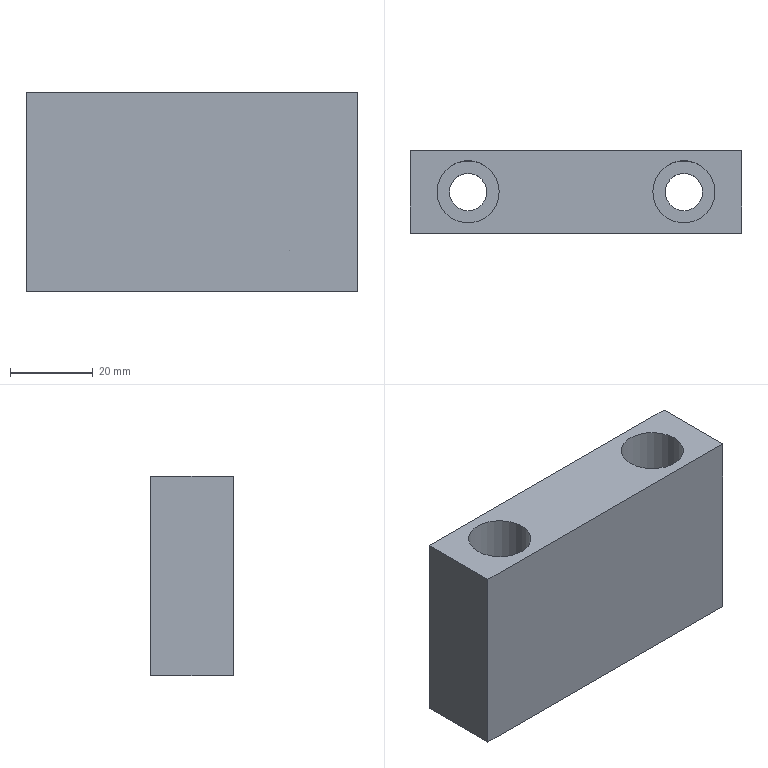Part | STEP file | gslz 2016.10.28-13_id498_x_t | 1 solid | 12 faces | box 80 x 20 x 48 mm | volume 65038 mm3 | plane 8 | cylinder 4 | commonest cylinder face diameters 9 x2 15 x2
STEP:
#1=CARTESIAN_POINT('',(0.,0.,0.));
#2=DIRECTION('',(0.,0.,1.));
#3=DIRECTION('',(1.,0.,0.));
#4=AXIS2_PLACEMENT_3D('',#1,#2,#3);
#5=CARTESIAN_POINT('',(-745.014,-46.466,0.));
#6=VERTEX_POINT('',#5);
#7=CARTESIAN_POINT('',(-737.514,-46.466,0.));
#8=DIRECTION('',(0.,0.,-1.));
#9=DIRECTION('',(-1.,0.,0.));
#10=AXIS2_PLACEMENT_3D('',#7,#8,#9);
#11=CIRCLE('',#10,7.5);
#12=CARTESIAN_POINT('',(-834.,82.556,0.));
#13=DIRECTION('',(0.,0.,-1.));
#14=DIRECTION('',(-1.,0.,0.));
#15=AXIS2_PLACEMENT_3D('',#12,#13,#14);
#16=PLANE('',#15);
#17=CARTESIAN_POINT('',(-96.486,-129.022));
#18=DIRECTION('',(1.,0.));
#19=AXIS2_PLACEMENT_2D('',#17,#18);
#20=CIRCLE('',#19,7.5);
#21=(GEOMETRIC_REPRESENTATION_CONTEXT(2)PARAMETRIC_REPRESENTATION_CONTEXT()REPRESENTATION_CONTEXT('',''));
#22=DEFINITIONAL_REPRESENTATION('',(#20),#21);
#23=PCURVE('',#16,#22);
#24=CARTESIAN_POINT('',(-737.514,-46.466,0.));
#25=DIRECTION('',(0.,0.,-1.));
#26=DIRECTION('',(-1.,0.,0.));
#27=AXIS2_PLACEMENT_3D('',#24,#25,#26);
#28=CYLINDRICAL_SURFACE('',#27,7.5);
#29=CARTESIAN_POINT('',(0.,0.));
#30=DIRECTION('',(1.,0.));
#31=VECTOR('',#30,1.);
#32=LINE('',#29,#31);
#33=(GEOMETRIC_REPRESENTATION_CONTEXT(2)PARAMETRIC_REPRESENTATION_CONTEXT()REPRESENTATION_CONTEXT('',''));
#34=DEFINITIONAL_REPRESENTATION('',(#32),#33);
#35=PCURVE('',#28,#34);
#36=SURFACE_CURVE('',#11,(#23,#35),.PCURVE_S1.);
#37=EDGE_CURVE('',#6,#6,#36,.T.);
#38=ORIENTED_EDGE('',*,*,#37,.T.);
#39=EDGE_LOOP('',(#38));
#40=FACE_BOUND('',#39,.T.);
#41=CARTESIAN_POINT('',(-797.014,-46.466,0.));
#42=VERTEX_POINT('',#41);
#43=CARTESIAN_POINT('',(-789.514,-46.466,0.));
#44=DIRECTION('',(0.,0.,-1.));
#45=DIRECTION('',(-1.,0.,0.));
#46=AXIS2_PLACEMENT_3D('',#43,#44,#45);
#47=CIRCLE('',#46,7.5);
#48=CARTESIAN_POINT('',(-44.486,-129.022));
#49=DIRECTION('',(1.,0.));
#50=AXIS2_PLACEMENT_2D('',#48,#49);
#51=CIRCLE('',#50,7.5);
#52=(GEOMETRIC_REPRESENTATION_CONTEXT(2)PARAMETRIC_REPRESENTATION_CONTEXT()REPRESENTATION_CONTEXT('',''));
#53=DEFINITIONAL_REPRESENTATION('',(#51),#52);
#54=PCURVE('',#16,#53);
#55=CARTESIAN_POINT('',(-789.514,-46.466,0.));
#56=DIRECTION('',(0.,0.,-1.));
#57=DIRECTION('',(-1.,0.,0.));
#58=AXIS2_PLACEMENT_3D('',#55,#56,#57);
#59=CYLINDRICAL_SURFACE('',#58,7.5);
#60=CARTESIAN_POINT('',(0.,0.));
#61=DIRECTION('',(1.,0.));
#62=VECTOR('',#61,1.);
#63=LINE('',#60,#62);
#64=(GEOMETRIC_REPRESENTATION_CONTEXT(2)PARAMETRIC_REPRESENTATION_CONTEXT()REPRESENTATION_CONTEXT('',''));
#65=DEFINITIONAL_REPRESENTATION('',(#63),#64);
#66=PCURVE('',#59,#65);
#67=SURFACE_CURVE('',#47,(#54,#66),.PCURVE_S1.);
#68=EDGE_CURVE('',#42,#42,#67,.T.);
#69=ORIENTED_EDGE('',*,*,#68,.T.);
#70=EDGE_LOOP('',(#69));
#71=FACE_BOUND('',#70,.T.);
#72=CARTESIAN_POINT('',(-723.514,-56.466,0.));
#73=VERTEX_POINT('',#72);
#74=CARTESIAN_POINT('',(-803.514,-56.466,0.));
#75=VERTEX_POINT('',#74);
#76=CARTESIAN_POINT('',(-763.514,-56.466,0.));
#77=DIRECTION('',(-1.,0.,0.));
#78=VECTOR('',#77,1.);
#79=LINE('',#76,#78);
#80=CARTESIAN_POINT('',(-70.486,-139.022));
#81=DIRECTION('',(1.,0.));
#82=VECTOR('',#81,1.);
#83=LINE('',#80,#82);
#84=(GEOMETRIC_REPRESENTATION_CONTEXT(2)PARAMETRIC_REPRESENTATION_CONTEXT()REPRESENTATION_CONTEXT('',''));
#85=DEFINITIONAL_REPRESENTATION('',(#83),#84);
#86=PCURVE('',#16,#85);
#87=CARTESIAN_POINT('',(-763.514,-56.466,-13.75));
#88=DIRECTION('',(0.,-1.,0.));
#89=DIRECTION('',(0.,0.,-1.));
#90=AXIS2_PLACEMENT_3D('',#87,#88,#89);
#91=PLANE('',#90);
#92=CARTESIAN_POINT('',(-13.75,0.));
#93=DIRECTION('',(0.,-1.));
#94=VECTOR('',#93,1.);
#95=LINE('',#92,#94);
#96=(GEOMETRIC_REPRESENTATION_CONTEXT(2)PARAMETRIC_REPRESENTATION_CONTEXT()REPRESENTATION_CONTEXT('',''));
#97=DEFINITIONAL_REPRESENTATION('',(#95),#96);
#98=PCURVE('',#91,#97);
#99=SURFACE_CURVE('',#79,(#86,#98),.PCURVE_S1.);
#100=EDGE_CURVE('',#73,#75,#99,.T.);
#101=ORIENTED_EDGE('',*,*,#100,.F.);
#102=CARTESIAN_POINT('',(-723.514,-36.466,0.));
#103=VERTEX_POINT('',#102);
#104=CARTESIAN_POINT('',(-723.514,-55.466,0.));
#105=DIRECTION('',(0.,-1.,0.));
#106=VECTOR('',#105,1.);
#107=LINE('',#104,#106);
#108=CARTESIAN_POINT('',(-110.486,-138.022));
#109=DIRECTION('',(0.,-1.));
#110=VECTOR('',#109,1.);
#111=LINE('',#108,#110);
#112=(GEOMETRIC_REPRESENTATION_CONTEXT(2)PARAMETRIC_REPRESENTATION_CONTEXT()REPRESENTATION_CONTEXT('',''));
#113=DEFINITIONAL_REPRESENTATION('',(#111),#112);
#114=PCURVE('',#16,#113);
#115=CARTESIAN_POINT('',(-723.514,-55.466,-13.75));
#116=DIRECTION('',(1.,0.,0.));
#117=DIRECTION('',(0.,0.,-1.));
#118=AXIS2_PLACEMENT_3D('',#115,#116,#117);
#119=PLANE('',#118);
#120=CARTESIAN_POINT('',(-13.75,0.));
#121=DIRECTION('',(0.,-1.));
#122=VECTOR('',#121,1.);
#123=LINE('',#120,#122);
#124=(GEOMETRIC_REPRESENTATION_CONTEXT(2)PARAMETRIC_REPRESENTATION_CONTEXT()REPRESENTATION_CONTEXT('',''));
#125=DEFINITIONAL_REPRESENTATION('',(#123),#124);
#126=PCURVE('',#119,#125);
#127=SURFACE_CURVE('',#107,(#114,#126),.PCURVE_S1.);
#128=EDGE_CURVE('',#103,#73,#127,.T.);
#129=ORIENTED_EDGE('',*,*,#128,.F.);
#130=CARTESIAN_POINT('',(-803.514,-36.466,0.));
#131=VERTEX_POINT('',#130);
#132=CARTESIAN_POINT('',(-763.514,-36.466,0.));
#133=DIRECTION('',(1.,0.,0.));
#134=VECTOR('',#133,1.);
#135=LINE('',#132,#134);
#136=CARTESIAN_POINT('',(-70.486,-119.022));
#137=DIRECTION('',(-1.,0.));
#138=VECTOR('',#137,1.);
#139=LINE('',#136,#138);
#140=(GEOMETRIC_REPRESENTATION_CONTEXT(2)PARAMETRIC_REPRESENTATION_CONTEXT()REPRESENTATION_CONTEXT('',''));
#141=DEFINITIONAL_REPRESENTATION('',(#139),#140);
#142=PCURVE('',#16,#141);
#143=CARTESIAN_POINT('',(-763.514,-36.466,-13.75));
#144=DIRECTION('',(0.,1.,0.));
#145=DIRECTION('',(0.,0.,1.));
#146=AXIS2_PLACEMENT_3D('',#143,#144,#145);
#147=PLANE('',#146);
#148=CARTESIAN_POINT('',(13.75,0.));
#149=DIRECTION('',(0.,1.));
#150=VECTOR('',#149,1.);
#151=LINE('',#148,#150);
#152=(GEOMETRIC_REPRESENTATION_CONTEXT(2)PARAMETRIC_REPRESENTATION_CONTEXT()REPRESENTATION_CONTEXT('',''));
#153=DEFINITIONAL_REPRESENTATION('',(#151),#152);
#154=PCURVE('',#147,#153);
#155=SURFACE_CURVE('',#135,(#142,#154),.PCURVE_S1.);
#156=EDGE_CURVE('',#131,#103,#155,.T.);
#157=ORIENTED_EDGE('',*,*,#156,.F.);
#158=CARTESIAN_POINT('',(-803.514,-55.466,0.));
#159=DIRECTION('',(0.,1.,0.));
#160=VECTOR('',#159,1.);
#161=LINE('',#158,#160);
#162=CARTESIAN_POINT('',(-30.486,-138.022));
#163=DIRECTION('',(0.,1.));
#164=VECTOR('',#163,1.);
#165=LINE('',#162,#164);
#166=(GEOMETRIC_REPRESENTATION_CONTEXT(2)PARAMETRIC_REPRESENTATION_CONTEXT()REPRESENTATION_CONTEXT('',''));
#167=DEFINITIONAL_REPRESENTATION('',(#165),#166);
#168=PCURVE('',#16,#167);
#169=CARTESIAN_POINT('',(-803.514,-55.466,-13.75));
#170=DIRECTION('',(-1.,0.,0.));
#171=DIRECTION('',(0.,0.,1.));
#172=AXIS2_PLACEMENT_3D('',#169,#170,#171);
#173=PLANE('',#172);
#174=CARTESIAN_POINT('',(13.75,0.));
#175=DIRECTION('',(0.,1.));
#176=VECTOR('',#175,1.);
#177=LINE('',#174,#176);
#178=(GEOMETRIC_REPRESENTATION_CONTEXT(2)PARAMETRIC_REPRESENTATION_CONTEXT()REPRESENTATION_CONTEXT('',''));
#179=DEFINITIONAL_REPRESENTATION('',(#177),#178);
#180=PCURVE('',#173,#179);
#181=SURFACE_CURVE('',#161,(#168,#180),.PCURVE_S1.);
#182=EDGE_CURVE('',#75,#131,#181,.T.);
#183=ORIENTED_EDGE('',*,*,#182,.F.);
#184=EDGE_LOOP('',(#101,#129,#157,#183));
#185=FACE_BOUND('',#184,.T.);
#186=ADVANCED_FACE('',(#40,#71,#185),#16,.F.);
#187=CARTESIAN_POINT('',(-723.514,-56.466,-48.));
#188=VERTEX_POINT('',#187);
#189=CARTESIAN_POINT('',(-723.514,-56.466,-13.75));
#190=DIRECTION('',(0.,0.,1.));
#191=VECTOR('',#190,1.);
#192=LINE('',#189,#191);
#193=CARTESIAN_POINT('',(0.,40.));
#194=DIRECTION('',(-1.,0.));
#195=VECTOR('',#194,1.);
#196=LINE('',#193,#195);
#197=(GEOMETRIC_REPRESENTATION_CONTEXT(2)PARAMETRIC_REPRESENTATION_CONTEXT()REPRESENTATION_CONTEXT('',''));
#198=DEFINITIONAL_REPRESENTATION('',(#196),#197);
#199=PCURVE('',#91,#198);
#200=CARTESIAN_POINT('',(0.,-1.));
#201=DIRECTION('',(-1.,0.));
#202=VECTOR('',#201,1.);
#203=LINE('',#200,#202);
#204=(GEOMETRIC_REPRESENTATION_CONTEXT(2)PARAMETRIC_REPRESENTATION_CONTEXT()REPRESENTATION_CONTEXT('',''));
#205=DEFINITIONAL_REPRESENTATION('',(#203),#204);
#206=PCURVE('',#119,#205);
#207=SURFACE_CURVE('',#192,(#199,#206),.PCURVE_S1.);
#208=EDGE_CURVE('',#188,#73,#207,.T.);
#209=ORIENTED_EDGE('',*,*,#208,.T.);
#210=ORIENTED_EDGE('',*,*,#100,.T.);
#211=CARTESIAN_POINT('',(-803.514,-56.466,-48.));
#212=VERTEX_POINT('',#211);
#213=CARTESIAN_POINT('',(-803.514,-56.466,-13.75));
#214=DIRECTION('',(0.,0.,1.));
#215=VECTOR('',#214,1.);
#216=LINE('',#213,#215);
#217=CARTESIAN_POINT('',(0.,-40.));
#218=DIRECTION('',(-1.,0.));
#219=VECTOR('',#218,1.);
#220=LINE('',#217,#219);
#221=(GEOMETRIC_REPRESENTATION_CONTEXT(2)PARAMETRIC_REPRESENTATION_CONTEXT()REPRESENTATION_CONTEXT('',''));
#222=DEFINITIONAL_REPRESENTATION('',(#220),#221);
#223=PCURVE('',#91,#222);
#224=CARTESIAN_POINT('',(0.,-1.));
#225=DIRECTION('',(1.,0.));
#226=VECTOR('',#225,1.);
#227=LINE('',#224,#226);
#228=(GEOMETRIC_REPRESENTATION_CONTEXT(2)PARAMETRIC_REPRESENTATION_CONTEXT()REPRESENTATION_CONTEXT('',''));
#229=DEFINITIONAL_REPRESENTATION('',(#227),#228);
#230=PCURVE('',#173,#229);
#231=SURFACE_CURVE('',#216,(#223,#230),.PCURVE_S1.);
#232=EDGE_CURVE('',#212,#75,#231,.T.);
#233=ORIENTED_EDGE('',*,*,#232,.F.);
#234=CARTESIAN_POINT('',(-763.514,-56.466,-48.));
#235=DIRECTION('',(1.,0.,0.));
#236=VECTOR('',#235,1.);
#237=LINE('',#234,#236);
#238=CARTESIAN_POINT('',(34.25,0.));
#239=DIRECTION('',(0.,1.));
#240=VECTOR('',#239,1.);
#241=LINE('',#238,#240);
#242=(GEOMETRIC_REPRESENTATION_CONTEXT(2)PARAMETRIC_REPRESENTATION_CONTEXT()REPRESENTATION_CONTEXT('',''));
#243=DEFINITIONAL_REPRESENTATION('',(#241),#242);
#244=PCURVE('',#91,#243);
#245=CARTESIAN_POINT('',(-834.,82.556,-48.));
#246=DIRECTION('',(0.,0.,-1.));
#247=DIRECTION('',(-1.,0.,0.));
#248=AXIS2_PLACEMENT_3D('',#245,#246,#247);
#249=PLANE('',#248);
#250=CARTESIAN_POINT('',(-70.486,-139.022));
#251=DIRECTION('',(-1.,0.));
#252=VECTOR('',#251,1.);
#253=LINE('',#250,#252);
#254=(GEOMETRIC_REPRESENTATION_CONTEXT(2)PARAMETRIC_REPRESENTATION_CONTEXT()REPRESENTATION_CONTEXT('',''));
#255=DEFINITIONAL_REPRESENTATION('',(#253),#254);
#256=PCURVE('',#249,#255);
#257=SURFACE_CURVE('',#237,(#244,#256),.PCURVE_S1.);
#258=EDGE_CURVE('',#212,#188,#257,.T.);
#259=ORIENTED_EDGE('',*,*,#258,.T.);
#260=EDGE_LOOP('',(#209,#210,#233,#259));
#261=FACE_BOUND('',#260,.T.);
#262=ADVANCED_FACE('',(#261),#91,.T.);
#263=ORIENTED_EDGE('',*,*,#232,.T.);
#264=ORIENTED_EDGE('',*,*,#182,.T.);
#265=CARTESIAN_POINT('',(-803.514,-36.466,-48.));
#266=VERTEX_POINT('',#265);
#267=CARTESIAN_POINT('',(-803.514,-36.466,-13.75));
#268=DIRECTION('',(0.,0.,1.));
#269=VECTOR('',#268,1.);
#270=LINE('',#267,#269);
#271=CARTESIAN_POINT('',(0.,19.));
#272=DIRECTION('',(1.,0.));
#273=VECTOR('',#272,1.);
#274=LINE('',#271,#273);
#275=(GEOMETRIC_REPRESENTATION_CONTEXT(2)PARAMETRIC_REPRESENTATION_CONTEXT()REPRESENTATION_CONTEXT('',''));
#276=DEFINITIONAL_REPRESENTATION('',(#274),#275);
#277=PCURVE('',#173,#276);
#278=CARTESIAN_POINT('',(0.,-40.));
#279=DIRECTION('',(1.,0.));
#280=VECTOR('',#279,1.);
#281=LINE('',#278,#280);
#282=(GEOMETRIC_REPRESENTATION_CONTEXT(2)PARAMETRIC_REPRESENTATION_CONTEXT()REPRESENTATION_CONTEXT('',''));
#283=DEFINITIONAL_REPRESENTATION('',(#281),#282);
#284=PCURVE('',#147,#283);
#285=SURFACE_CURVE('',#270,(#277,#284),.PCURVE_S1.);
#286=EDGE_CURVE('',#266,#131,#285,.T.);
#287=ORIENTED_EDGE('',*,*,#286,.F.);
#288=CARTESIAN_POINT('',(-803.514,-55.466,-48.));
#289=DIRECTION('',(0.,-1.,0.));
#290=VECTOR('',#289,1.);
#291=LINE('',#288,#290);
#292=CARTESIAN_POINT('',(-34.25,0.));
#293=DIRECTION('',(0.,-1.));
#294=VECTOR('',#293,1.);
#295=LINE('',#292,#294);
#296=(GEOMETRIC_REPRESENTATION_CONTEXT(2)PARAMETRIC_REPRESENTATION_CONTEXT()REPRESENTATION_CONTEXT('',''));
#297=DEFINITIONAL_REPRESENTATION('',(#295),#296);
#298=PCURVE('',#173,#297);
#299=CARTESIAN_POINT('',(-30.486,-138.022));
#300=DIRECTION('',(0.,-1.));
#301=VECTOR('',#300,1.);
#302=LINE('',#299,#301);
#303=(GEOMETRIC_REPRESENTATION_CONTEXT(2)PARAMETRIC_REPRESENTATION_CONTEXT()REPRESENTATION_CONTEXT('',''));
#304=DEFINITIONAL_REPRESENTATION('',(#302),#303);
#305=PCURVE('',#249,#304);
#306=SURFACE_CURVE('',#291,(#298,#305),.PCURVE_S1.);
#307=EDGE_CURVE('',#266,#212,#306,.T.);
#308=ORIENTED_EDGE('',*,*,#307,.T.);
#309=EDGE_LOOP('',(#263,#264,#287,#308));
#310=FACE_BOUND('',#309,.T.);
#311=ADVANCED_FACE('',(#310),#173,.T.);
#312=ORIENTED_EDGE('',*,*,#286,.T.);
#313=ORIENTED_EDGE('',*,*,#156,.T.);
#314=CARTESIAN_POINT('',(-723.514,-36.466,-48.));
#315=VERTEX_POINT('',#314);
#316=CARTESIAN_POINT('',(-723.514,-36.466,-13.75));
#317=DIRECTION('',(0.,0.,1.));
#318=VECTOR('',#317,1.);
#319=LINE('',#316,#318);
#320=CARTESIAN_POINT('',(0.,40.));
#321=DIRECTION('',(1.,0.));
#322=VECTOR('',#321,1.);
#323=LINE('',#320,#322);
#324=(GEOMETRIC_REPRESENTATION_CONTEXT(2)PARAMETRIC_REPRESENTATION_CONTEXT()REPRESENTATION_CONTEXT('',''));
#325=DEFINITIONAL_REPRESENTATION('',(#323),#324);
#326=PCURVE('',#147,#325);
#327=CARTESIAN_POINT('',(0.,19.));
#328=DIRECTION('',(-1.,0.));
#329=VECTOR('',#328,1.);
#330=LINE('',#327,#329);
#331=(GEOMETRIC_REPRESENTATION_CONTEXT(2)PARAMETRIC_REPRESENTATION_CONTEXT()REPRESENTATION_CONTEXT('',''));
#332=DEFINITIONAL_REPRESENTATION('',(#330),#331);
#333=PCURVE('',#119,#332);
#334=SURFACE_CURVE('',#319,(#326,#333),.PCURVE_S1.);
#335=EDGE_CURVE('',#315,#103,#334,.T.);
#336=ORIENTED_EDGE('',*,*,#335,.F.);
#337=CARTESIAN_POINT('',(-763.514,-36.466,-48.));
#338=DIRECTION('',(-1.,0.,0.));
#339=VECTOR('',#338,1.);
#340=LINE('',#337,#339);
#341=CARTESIAN_POINT('',(-34.25,0.));
#342=DIRECTION('',(0.,-1.));
#343=VECTOR('',#342,1.);
#344=LINE('',#341,#343);
#345=(GEOMETRIC_REPRESENTATION_CONTEXT(2)PARAMETRIC_REPRESENTATION_CONTEXT()REPRESENTATION_CONTEXT('',''));
#346=DEFINITIONAL_REPRESENTATION('',(#344),#345);
#347=PCURVE('',#147,#346);
#348=CARTESIAN_POINT('',(-70.486,-119.022));
#349=DIRECTION('',(1.,0.));
#350=VECTOR('',#349,1.);
#351=LINE('',#348,#350);
#352=(GEOMETRIC_REPRESENTATION_CONTEXT(2)PARAMETRIC_REPRESENTATION_CONTEXT()REPRESENTATION_CONTEXT('',''));
#353=DEFINITIONAL_REPRESENTATION('',(#351),#352);
#354=PCURVE('',#249,#353);
#355=SURFACE_CURVE('',#340,(#347,#354),.PCURVE_S1.);
#356=EDGE_CURVE('',#315,#266,#355,.T.);
#357=ORIENTED_EDGE('',*,*,#356,.T.);
#358=EDGE_LOOP('',(#312,#313,#336,#357));
#359=FACE_BOUND('',#358,.T.);
#360=ADVANCED_FACE('',(#359),#147,.T.);
#361=CARTESIAN_POINT('',(-742.014,-46.466,-48.));
#362=VERTEX_POINT('',#361);
#363=CARTESIAN_POINT('',(-737.514,-46.466,-48.));
#364=DIRECTION('',(0.,0.,-1.));
#365=DIRECTION('',(-1.,0.,0.));
#366=AXIS2_PLACEMENT_3D('',#363,#364,#365);
#367=CIRCLE('',#366,4.5);
#368=CARTESIAN_POINT('',(-96.486,-129.022));
#369=DIRECTION('',(1.,0.));
#370=AXIS2_PLACEMENT_2D('',#368,#369);
#371=CIRCLE('',#370,4.5);
#372=(GEOMETRIC_REPRESENTATION_CONTEXT(2)PARAMETRIC_REPRESENTATION_CONTEXT()REPRESENTATION_CONTEXT('',''));
#373=DEFINITIONAL_REPRESENTATION('',(#371),#372);
#374=PCURVE('',#249,#373);
#375=CARTESIAN_POINT('',(-737.514,-46.466,-150.));
#376=DIRECTION('',(0.,0.,-1.));
#377=DIRECTION('',(-1.,0.,0.));
#378=AXIS2_PLACEMENT_3D('',#375,#376,#377);
#379=CYLINDRICAL_SURFACE('',#378,4.5);
#380=CARTESIAN_POINT('',(0.,-102.));
#381=DIRECTION('',(1.,0.));
#382=VECTOR('',#381,1.);
#383=LINE('',#380,#382);
#384=(GEOMETRIC_REPRESENTATION_CONTEXT(2)PARAMETRIC_REPRESENTATION_CONTEXT()REPRESENTATION_CONTEXT('',''));
#385=DEFINITIONAL_REPRESENTATION('',(#383),#384);
#386=PCURVE('',#379,#385);
#387=SURFACE_CURVE('',#367,(#374,#386),.PCURVE_S1.);
#388=EDGE_CURVE('',#362,#362,#387,.T.);
#389=ORIENTED_EDGE('',*,*,#388,.F.);
#390=EDGE_LOOP('',(#389));
#391=FACE_BOUND('',#390,.T.);
#392=CARTESIAN_POINT('',(-794.014,-46.466,-48.));
#393=VERTEX_POINT('',#392);
#394=CARTESIAN_POINT('',(-789.514,-46.466,-48.));
#395=DIRECTION('',(0.,0.,-1.));
#396=DIRECTION('',(-1.,0.,0.));
#397=AXIS2_PLACEMENT_3D('',#394,#395,#396);
#398=CIRCLE('',#397,4.5);
#399=CARTESIAN_POINT('',(-44.486,-129.022));
#400=DIRECTION('',(1.,0.));
#401=AXIS2_PLACEMENT_2D('',#399,#400);
#402=CIRCLE('',#401,4.5);
#403=(GEOMETRIC_REPRESENTATION_CONTEXT(2)PARAMETRIC_REPRESENTATION_CONTEXT()REPRESENTATION_CONTEXT('',''));
#404=DEFINITIONAL_REPRESENTATION('',(#402),#403);
#405=PCURVE('',#249,#404);
#406=CARTESIAN_POINT('',(-789.514,-46.466,-150.));
#407=DIRECTION('',(0.,0.,-1.));
#408=DIRECTION('',(-1.,0.,0.));
#409=AXIS2_PLACEMENT_3D('',#406,#407,#408);
#410=CYLINDRICAL_SURFACE('',#409,4.5);
#411=CARTESIAN_POINT('',(0.,-102.));
#412=DIRECTION('',(1.,0.));
#413=VECTOR('',#412,1.);
#414=LINE('',#411,#413);
#415=(GEOMETRIC_REPRESENTATION_CONTEXT(2)PARAMETRIC_REPRESENTATION_CONTEXT()REPRESENTATION_CONTEXT('',''));
#416=DEFINITIONAL_REPRESENTATION('',(#414),#415);
#417=PCURVE('',#410,#416);
#418=SURFACE_CURVE('',#398,(#405,#417),.PCURVE_S1.);
#419=EDGE_CURVE('',#393,#393,#418,.T.);
#420=ORIENTED_EDGE('',*,*,#419,.F.);
#421=EDGE_LOOP('',(#420));
#422=FACE_BOUND('',#421,.T.);
#423=CARTESIAN_POINT('',(-723.514,-55.466,-48.));
#424=DIRECTION('',(0.,1.,0.));
#425=VECTOR('',#424,1.);
#426=LINE('',#423,#425);
#427=CARTESIAN_POINT('',(-110.486,-138.022));
#428=DIRECTION('',(0.,1.));
#429=VECTOR('',#428,1.);
#430=LINE('',#427,#429);
#431=(GEOMETRIC_REPRESENTATION_CONTEXT(2)PARAMETRIC_REPRESENTATION_CONTEXT()REPRESENTATION_CONTEXT('',''));
#432=DEFINITIONAL_REPRESENTATION('',(#430),#431);
#433=PCURVE('',#249,#432);
#434=CARTESIAN_POINT('',(34.25,0.));
#435=DIRECTION('',(0.,1.));
#436=VECTOR('',#435,1.);
#437=LINE('',#434,#436);
#438=(GEOMETRIC_REPRESENTATION_CONTEXT(2)PARAMETRIC_REPRESENTATION_CONTEXT()REPRESENTATION_CONTEXT('',''));
#439=DEFINITIONAL_REPRESENTATION('',(#437),#438);
#440=PCURVE('',#119,#439);
#441=SURFACE_CURVE('',#426,(#433,#440),.PCURVE_S1.);
#442=EDGE_CURVE('',#188,#315,#441,.T.);
#443=ORIENTED_EDGE('',*,*,#442,.F.);
#444=ORIENTED_EDGE('',*,*,#258,.F.);
#445=ORIENTED_EDGE('',*,*,#307,.F.);
#446=ORIENTED_EDGE('',*,*,#356,.F.);
#447=EDGE_LOOP('',(#443,#444,#445,#446));
#448=FACE_BOUND('',#447,.T.);
#449=ADVANCED_FACE('',(#391,#422,#448),#249,.T.);
#450=ORIENTED_EDGE('',*,*,#442,.T.);
#451=ORIENTED_EDGE('',*,*,#335,.T.);
#452=ORIENTED_EDGE('',*,*,#128,.T.);
#453=ORIENTED_EDGE('',*,*,#208,.F.);
#454=EDGE_LOOP('',(#450,#451,#452,#453));
#455=FACE_BOUND('',#454,.T.);
#456=ADVANCED_FACE('',(#455),#119,.T.);
#457=ORIENTED_EDGE('',*,*,#419,.F.);
#458=CARTESIAN_POINT('',(-794.014,-46.466,-25.));
#459=VERTEX_POINT('',#458);
#460=CARTESIAN_POINT('',(-794.014,-46.466,-25.));
#461=CARTESIAN_POINT('',(-794.014,-46.466,-48.));
#462=B_SPLINE_CURVE_WITH_KNOTS('',1,(#460,#461),.UNSPECIFIED.,.F.,.F.,(2,2),(-125.,-102.),.PIECEWISE_BEZIER_KNOTS.);
#463=CARTESIAN_POINT('',(0.,0.));
#464=DIRECTION('',(0.,1.));
#465=VECTOR('',#464,1.);
#466=LINE('',#463,#465);
#467=(GEOMETRIC_REPRESENTATION_CONTEXT(2)PARAMETRIC_REPRESENTATION_CONTEXT()REPRESENTATION_CONTEXT('',''));
#468=DEFINITIONAL_REPRESENTATION('',(#466),#467);
#469=PCURVE('',#410,#468);
#470=CARTESIAN_POINT('',(6.283,0.));
#471=DIRECTION('',(0.,1.));
#472=VECTOR('',#471,1.);
#473=LINE('',#470,#472);
#474=(GEOMETRIC_REPRESENTATION_CONTEXT(2)PARAMETRIC_REPRESENTATION_CONTEXT()REPRESENTATION_CONTEXT('',''));
#475=DEFINITIONAL_REPRESENTATION('',(#473),#474);
#476=PCURVE('',#410,#475);
#477=SEAM_CURVE('',#462,(#469,#476),.PCURVE_S1.);
#478=EDGE_CURVE('',#459,#393,#477,.T.);
#479=ORIENTED_EDGE('',*,*,#478,.F.);
#480=CARTESIAN_POINT('',(-789.514,-46.466,-25.));
#481=DIRECTION('',(0.,0.,1.));
#482=DIRECTION('',(-1.,0.,0.));
#483=AXIS2_PLACEMENT_3D('',#480,#481,#482);
#484=CIRCLE('',#483,4.5);
#485=CARTESIAN_POINT('',(6.283,-125.));
#486=DIRECTION('',(-1.,0.));
#487=VECTOR('',#486,1.);
#488=LINE('',#485,#487);
#489=(GEOMETRIC_REPRESENTATION_CONTEXT(2)PARAMETRIC_REPRESENTATION_CONTEXT()REPRESENTATION_CONTEXT('',''));
#490=DEFINITIONAL_REPRESENTATION('',(#488),#489);
#491=PCURVE('',#410,#490);
#492=CARTESIAN_POINT('',(-789.514,-46.466,-25.));
#493=DIRECTION('',(0.,0.,-1.));
#494=DIRECTION('',(-1.,0.,0.));
#495=AXIS2_PLACEMENT_3D('',#492,#493,#494);
#496=PLANE('',#495);
#497=CARTESIAN_POINT('',(4.5,0.));
#498=CARTESIAN_POINT('',(4.5,-7.794));
#499=CARTESIAN_POINT('',(-2.25,-3.897));
#500=CARTESIAN_POINT('',(-9.,0.));
#501=CARTESIAN_POINT('',(-2.25,3.897));
#502=CARTESIAN_POINT('',(4.5,7.794));
#503=CARTESIAN_POINT('',(4.5,0.));
#504=(BOUNDED_CURVE()B_SPLINE_CURVE(2,(#497,#498,#499,#500,#501,#502,#503),.UNSPECIFIED.,.T.,.F.)B_SPLINE_CURVE_WITH_KNOTS((1,2,2,2,2,1),(-2.094,0.,2.094,4.189,6.283,8.378),.UNSPECIFIED.)CURVE()GEOMETRIC_REPRESENTATION_ITEM()RATIONAL_B_SPLINE_CURVE((1.,0.5,1.,0.5,1.,0.5,1.))REPRESENTATION_ITEM(''));
#505=(GEOMETRIC_REPRESENTATION_CONTEXT(2)PARAMETRIC_REPRESENTATION_CONTEXT()REPRESENTATION_CONTEXT('',''));
#506=DEFINITIONAL_REPRESENTATION('',(#504),#505);
#507=PCURVE('',#496,#506);
#508=SURFACE_CURVE('',#484,(#491,#507),.PCURVE_S1.);
#509=EDGE_CURVE('',#459,#459,#508,.T.);
#510=ORIENTED_EDGE('',*,*,#509,.F.);
#511=ORIENTED_EDGE('',*,*,#478,.T.);
#512=EDGE_LOOP('',(#457,#479,#510,#511));
#513=FACE_BOUND('',#512,.F.);
#514=ADVANCED_FACE('',(#513),#410,.F.);
#515=ORIENTED_EDGE('',*,*,#509,.F.);
#516=EDGE_LOOP('',(#515));
#517=FACE_BOUND('',#516,.T.);
#518=CARTESIAN_POINT('',(-797.014,-46.466,-25.));
#519=VERTEX_POINT('',#518);
#520=CARTESIAN_POINT('',(-789.514,-46.466,-25.));
#521=DIRECTION('',(0.,0.,1.));
#522=DIRECTION('',(-1.,0.,0.));
#523=AXIS2_PLACEMENT_3D('',#520,#521,#522);
#524=CIRCLE('',#523,7.5);
#525=CARTESIAN_POINT('',(7.5,0.));
#526=CARTESIAN_POINT('',(7.5,-12.99));
#527=CARTESIAN_POINT('',(-3.75,-6.495));
#528=CARTESIAN_POINT('',(-15.,0.));
#529=CARTESIAN_POINT('',(-3.75,6.495));
#530=CARTESIAN_POINT('',(7.5,12.99));
#531=CARTESIAN_POINT('',(7.5,0.));
#532=(BOUNDED_CURVE()B_SPLINE_CURVE(2,(#525,#526,#527,#528,#529,#530,#531),.UNSPECIFIED.,.T.,.F.)B_SPLINE_CURVE_WITH_KNOTS((1,2,2,2,2,1),(-2.094,0.,2.094,4.189,6.283,8.378),.UNSPECIFIED.)CURVE()GEOMETRIC_REPRESENTATION_ITEM()RATIONAL_B_SPLINE_CURVE((1.,0.5,1.,0.5,1.,0.5,1.))REPRESENTATION_ITEM(''));
#533=(GEOMETRIC_REPRESENTATION_CONTEXT(2)PARAMETRIC_REPRESENTATION_CONTEXT()REPRESENTATION_CONTEXT('',''));
#534=DEFINITIONAL_REPRESENTATION('',(#532),#533);
#535=PCURVE('',#496,#534);
#536=CARTESIAN_POINT('',(6.283,25.));
#537=DIRECTION('',(-1.,0.));
#538=VECTOR('',#537,1.);
#539=LINE('',#536,#538);
#540=(GEOMETRIC_REPRESENTATION_CONTEXT(2)PARAMETRIC_REPRESENTATION_CONTEXT()REPRESENTATION_CONTEXT('',''));
#541=DEFINITIONAL_REPRESENTATION('',(#539),#540);
#542=PCURVE('',#59,#541);
#543=SURFACE_CURVE('',#524,(#535,#542),.PCURVE_S1.);
#544=EDGE_CURVE('',#519,#519,#543,.T.);
#545=ORIENTED_EDGE('',*,*,#544,.T.);
#546=EDGE_LOOP('',(#545));
#547=FACE_BOUND('',#546,.T.);
#548=ADVANCED_FACE('',(#517,#547),#496,.F.);
#549=ORIENTED_EDGE('',*,*,#544,.T.);
#550=CARTESIAN_POINT('',(-797.014,-46.466,0.));
#551=CARTESIAN_POINT('',(-797.014,-46.466,-25.));
#552=B_SPLINE_CURVE_WITH_KNOTS('',1,(#550,#551),.UNSPECIFIED.,.F.,.F.,(2,2),(0.,25.),.PIECEWISE_BEZIER_KNOTS.);
#553=CARTESIAN_POINT('',(0.,0.));
#554=DIRECTION('',(0.,1.));
#555=VECTOR('',#554,1.);
#556=LINE('',#553,#555);
#557=(GEOMETRIC_REPRESENTATION_CONTEXT(2)PARAMETRIC_REPRESENTATION_CONTEXT()REPRESENTATION_CONTEXT('',''));
#558=DEFINITIONAL_REPRESENTATION('',(#556),#557);
#559=PCURVE('',#59,#558);
#560=CARTESIAN_POINT('',(6.283,0.));
#561=DIRECTION('',(0.,1.));
#562=VECTOR('',#561,1.);
#563=LINE('',#560,#562);
#564=(GEOMETRIC_REPRESENTATION_CONTEXT(2)PARAMETRIC_REPRESENTATION_CONTEXT()REPRESENTATION_CONTEXT('',''));
#565=DEFINITIONAL_REPRESENTATION('',(#563),#564);
#566=PCURVE('',#59,#565);
#567=SEAM_CURVE('',#552,(#559,#566),.PCURVE_S1.);
#568=EDGE_CURVE('',#42,#519,#567,.T.);
#569=ORIENTED_EDGE('',*,*,#568,.F.);
#570=ORIENTED_EDGE('',*,*,#68,.T.);
#571=ORIENTED_EDGE('',*,*,#568,.T.);
#572=EDGE_LOOP('',(#549,#569,#570,#571));
#573=FACE_BOUND('',#572,.F.);
#574=ADVANCED_FACE('',(#573),#59,.F.);
#575=ORIENTED_EDGE('',*,*,#388,.F.);
#576=CARTESIAN_POINT('',(-742.014,-46.466,-25.));
#577=VERTEX_POINT('',#576);
#578=CARTESIAN_POINT('',(-742.014,-46.466,-25.));
#579=CARTESIAN_POINT('',(-742.014,-46.466,-48.));
#580=B_SPLINE_CURVE_WITH_KNOTS('',1,(#578,#579),.UNSPECIFIED.,.F.,.F.,(2,2),(-125.,-102.),.PIECEWISE_BEZIER_KNOTS.);
#581=CARTESIAN_POINT('',(0.,0.));
#582=DIRECTION('',(0.,1.));
#583=VECTOR('',#582,1.);
#584=LINE('',#581,#583);
#585=(GEOMETRIC_REPRESENTATION_CONTEXT(2)PARAMETRIC_REPRESENTATION_CONTEXT()REPRESENTATION_CONTEXT('',''));
#586=DEFINITIONAL_REPRESENTATION('',(#584),#585);
#587=PCURVE('',#379,#586);
#588=CARTESIAN_POINT('',(6.283,0.));
#589=DIRECTION('',(0.,1.));
#590=VECTOR('',#589,1.);
#591=LINE('',#588,#590);
#592=(GEOMETRIC_REPRESENTATION_CONTEXT(2)PARAMETRIC_REPRESENTATION_CONTEXT()REPRESENTATION_CONTEXT('',''));
#593=DEFINITIONAL_REPRESENTATION('',(#591),#592);
#594=PCURVE('',#379,#593);
#595=SEAM_CURVE('',#580,(#587,#594),.PCURVE_S1.);
#596=EDGE_CURVE('',#577,#362,#595,.T.);
#597=ORIENTED_EDGE('',*,*,#596,.F.);
#598=CARTESIAN_POINT('',(-737.514,-46.466,-25.));
#599=DIRECTION('',(0.,0.,1.));
#600=DIRECTION('',(-1.,0.,0.));
#601=AXIS2_PLACEMENT_3D('',#598,#599,#600);
#602=CIRCLE('',#601,4.5);
#603=CARTESIAN_POINT('',(6.283,-125.));
#604=DIRECTION('',(-1.,0.));
#605=VECTOR('',#604,1.);
#606=LINE('',#603,#605);
#607=(GEOMETRIC_REPRESENTATION_CONTEXT(2)PARAMETRIC_REPRESENTATION_CONTEXT()REPRESENTATION_CONTEXT('',''));
#608=DEFINITIONAL_REPRESENTATION('',(#606),#607);
#609=PCURVE('',#379,#608);
#610=CARTESIAN_POINT('',(-737.514,-46.466,-25.));
#611=DIRECTION('',(0.,0.,-1.));
#612=DIRECTION('',(-1.,0.,0.));
#613=AXIS2_PLACEMENT_3D('',#610,#611,#612);
#614=PLANE('',#613);
#615=CARTESIAN_POINT('',(4.5,0.));
#616=CARTESIAN_POINT('',(4.5,-7.794));
#617=CARTESIAN_POINT('',(-2.25,-3.897));
#618=CARTESIAN_POINT('',(-9.,0.));
#619=CARTESIAN_POINT('',(-2.25,3.897));
#620=CARTESIAN_POINT('',(4.5,7.794));
#621=CARTESIAN_POINT('',(4.5,0.));
#622=(BOUNDED_CURVE()B_SPLINE_CURVE(2,(#615,#616,#617,#618,#619,#620,#621),.UNSPECIFIED.,.T.,.F.)B_SPLINE_CURVE_WITH_KNOTS((1,2,2,2,2,1),(-2.094,0.,2.094,4.189,6.283,8.378),.UNSPECIFIED.)CURVE()GEOMETRIC_REPRESENTATION_ITEM()RATIONAL_B_SPLINE_CURVE((1.,0.5,1.,0.5,1.,0.5,1.))REPRESENTATION_ITEM(''));
#623=(GEOMETRIC_REPRESENTATION_CONTEXT(2)PARAMETRIC_REPRESENTATION_CONTEXT()REPRESENTATION_CONTEXT('',''));
#624=DEFINITIONAL_REPRESENTATION('',(#622),#623);
#625=PCURVE('',#614,#624);
#626=SURFACE_CURVE('',#602,(#609,#625),.PCURVE_S1.);
#627=EDGE_CURVE('',#577,#577,#626,.T.);
#628=ORIENTED_EDGE('',*,*,#627,.F.);
#629=ORIENTED_EDGE('',*,*,#596,.T.);
#630=EDGE_LOOP('',(#575,#597,#628,#629));
#631=FACE_BOUND('',#630,.F.);
#632=ADVANCED_FACE('',(#631),#379,.F.);
#633=ORIENTED_EDGE('',*,*,#627,.F.);
#634=EDGE_LOOP('',(#633));
#635=FACE_BOUND('',#634,.T.);
#636=CARTESIAN_POINT('',(-745.014,-46.466,-25.));
#637=VERTEX_POINT('',#636);
#638=CARTESIAN_POINT('',(-737.514,-46.466,-25.));
#639=DIRECTION('',(0.,0.,1.));
#640=DIRECTION('',(-1.,0.,0.));
#641=AXIS2_PLACEMENT_3D('',#638,#639,#640);
#642=CIRCLE('',#641,7.5);
#643=CARTESIAN_POINT('',(7.5,0.));
#644=CARTESIAN_POINT('',(7.5,-12.99));
#645=CARTESIAN_POINT('',(-3.75,-6.495));
#646=CARTESIAN_POINT('',(-15.,0.));
#647=CARTESIAN_POINT('',(-3.75,6.495));
#648=CARTESIAN_POINT('',(7.5,12.99));
#649=CARTESIAN_POINT('',(7.5,0.));
#650=(BOUNDED_CURVE()B_SPLINE_CURVE(2,(#643,#644,#645,#646,#647,#648,#649),.UNSPECIFIED.,.T.,.F.)B_SPLINE_CURVE_WITH_KNOTS((1,2,2,2,2,1),(-2.094,0.,2.094,4.189,6.283,8.378),.UNSPECIFIED.)CURVE()GEOMETRIC_REPRESENTATION_ITEM()RATIONAL_B_SPLINE_CURVE((1.,0.5,1.,0.5,1.,0.5,1.))REPRESENTATION_ITEM(''));
#651=(GEOMETRIC_REPRESENTATION_CONTEXT(2)PARAMETRIC_REPRESENTATION_CONTEXT()REPRESENTATION_CONTEXT('',''));
#652=DEFINITIONAL_REPRESENTATION('',(#650),#651);
#653=PCURVE('',#614,#652);
#654=CARTESIAN_POINT('',(6.283,25.));
#655=DIRECTION('',(-1.,0.));
#656=VECTOR('',#655,1.);
#657=LINE('',#654,#656);
#658=(GEOMETRIC_REPRESENTATION_CONTEXT(2)PARAMETRIC_REPRESENTATION_CONTEXT()REPRESENTATION_CONTEXT('',''));
#659=DEFINITIONAL_REPRESENTATION('',(#657),#658);
#660=PCURVE('',#28,#659);
#661=SURFACE_CURVE('',#642,(#653,#660),.PCURVE_S1.);
#662=EDGE_CURVE('',#637,#637,#661,.T.);
#663=ORIENTED_EDGE('',*,*,#662,.T.);
#664=EDGE_LOOP('',(#663));
#665=FACE_BOUND('',#664,.T.);
#666=ADVANCED_FACE('',(#635,#665),#614,.F.);
#667=ORIENTED_EDGE('',*,*,#662,.T.);
#668=CARTESIAN_POINT('',(-745.014,-46.466,0.));
#669=CARTESIAN_POINT('',(-745.014,-46.466,-25.));
#670=B_SPLINE_CURVE_WITH_KNOTS('',1,(#668,#669),.UNSPECIFIED.,.F.,.F.,(2,2),(0.,25.),.PIECEWISE_BEZIER_KNOTS.);
#671=CARTESIAN_POINT('',(0.,0.));
#672=DIRECTION('',(0.,1.));
#673=VECTOR('',#672,1.);
#674=LINE('',#671,#673);
#675=(GEOMETRIC_REPRESENTATION_CONTEXT(2)PARAMETRIC_REPRESENTATION_CONTEXT()REPRESENTATION_CONTEXT('',''));
#676=DEFINITIONAL_REPRESENTATION('',(#674),#675);
#677=PCURVE('',#28,#676);
#678=CARTESIAN_POINT('',(6.283,0.));
#679=DIRECTION('',(0.,1.));
#680=VECTOR('',#679,1.);
#681=LINE('',#678,#680);
#682=(GEOMETRIC_REPRESENTATION_CONTEXT(2)PARAMETRIC_REPRESENTATION_CONTEXT()REPRESENTATION_CONTEXT('',''));
#683=DEFINITIONAL_REPRESENTATION('',(#681),#682);
#684=PCURVE('',#28,#683);
#685=SEAM_CURVE('',#670,(#677,#684),.PCURVE_S1.);
#686=EDGE_CURVE('',#6,#637,#685,.T.);
#687=ORIENTED_EDGE('',*,*,#686,.F.);
#688=ORIENTED_EDGE('',*,*,#37,.T.);
#689=ORIENTED_EDGE('',*,*,#686,.T.);
#690=EDGE_LOOP('',(#667,#687,#688,#689));
#691=FACE_BOUND('',#690,.F.);
#692=ADVANCED_FACE('',(#691),#28,.F.);
#693=CLOSED_SHELL('',(#186,#262,#311,#360,#449,#456,#514,#548,#574,#632,#666,#692));
#694=MANIFOLD_SOLID_BREP('',#693);
#695=(LENGTH_UNIT()NAMED_UNIT(*)SI_UNIT(.MILLI.,.METRE.));
#696=UNCERTAINTY_MEASURE_WITH_UNIT(LENGTH_MEASURE(0.000005),#695,'','');
#697=(NAMED_UNIT(*)PLANE_ANGLE_UNIT()SI_UNIT($,.RADIAN.));
#698=(NAMED_UNIT(*)SI_UNIT($,.STERADIAN.)SOLID_ANGLE_UNIT());
#699=(GEOMETRIC_REPRESENTATION_CONTEXT(3)GLOBAL_UNCERTAINTY_ASSIGNED_CONTEXT((#696))GLOBAL_UNIT_ASSIGNED_CONTEXT((#695,#697,#698))REPRESENTATION_CONTEXT('',''));
#700=ADVANCED_BREP_SHAPE_REPRESENTATION('',(#4,#694),#699);